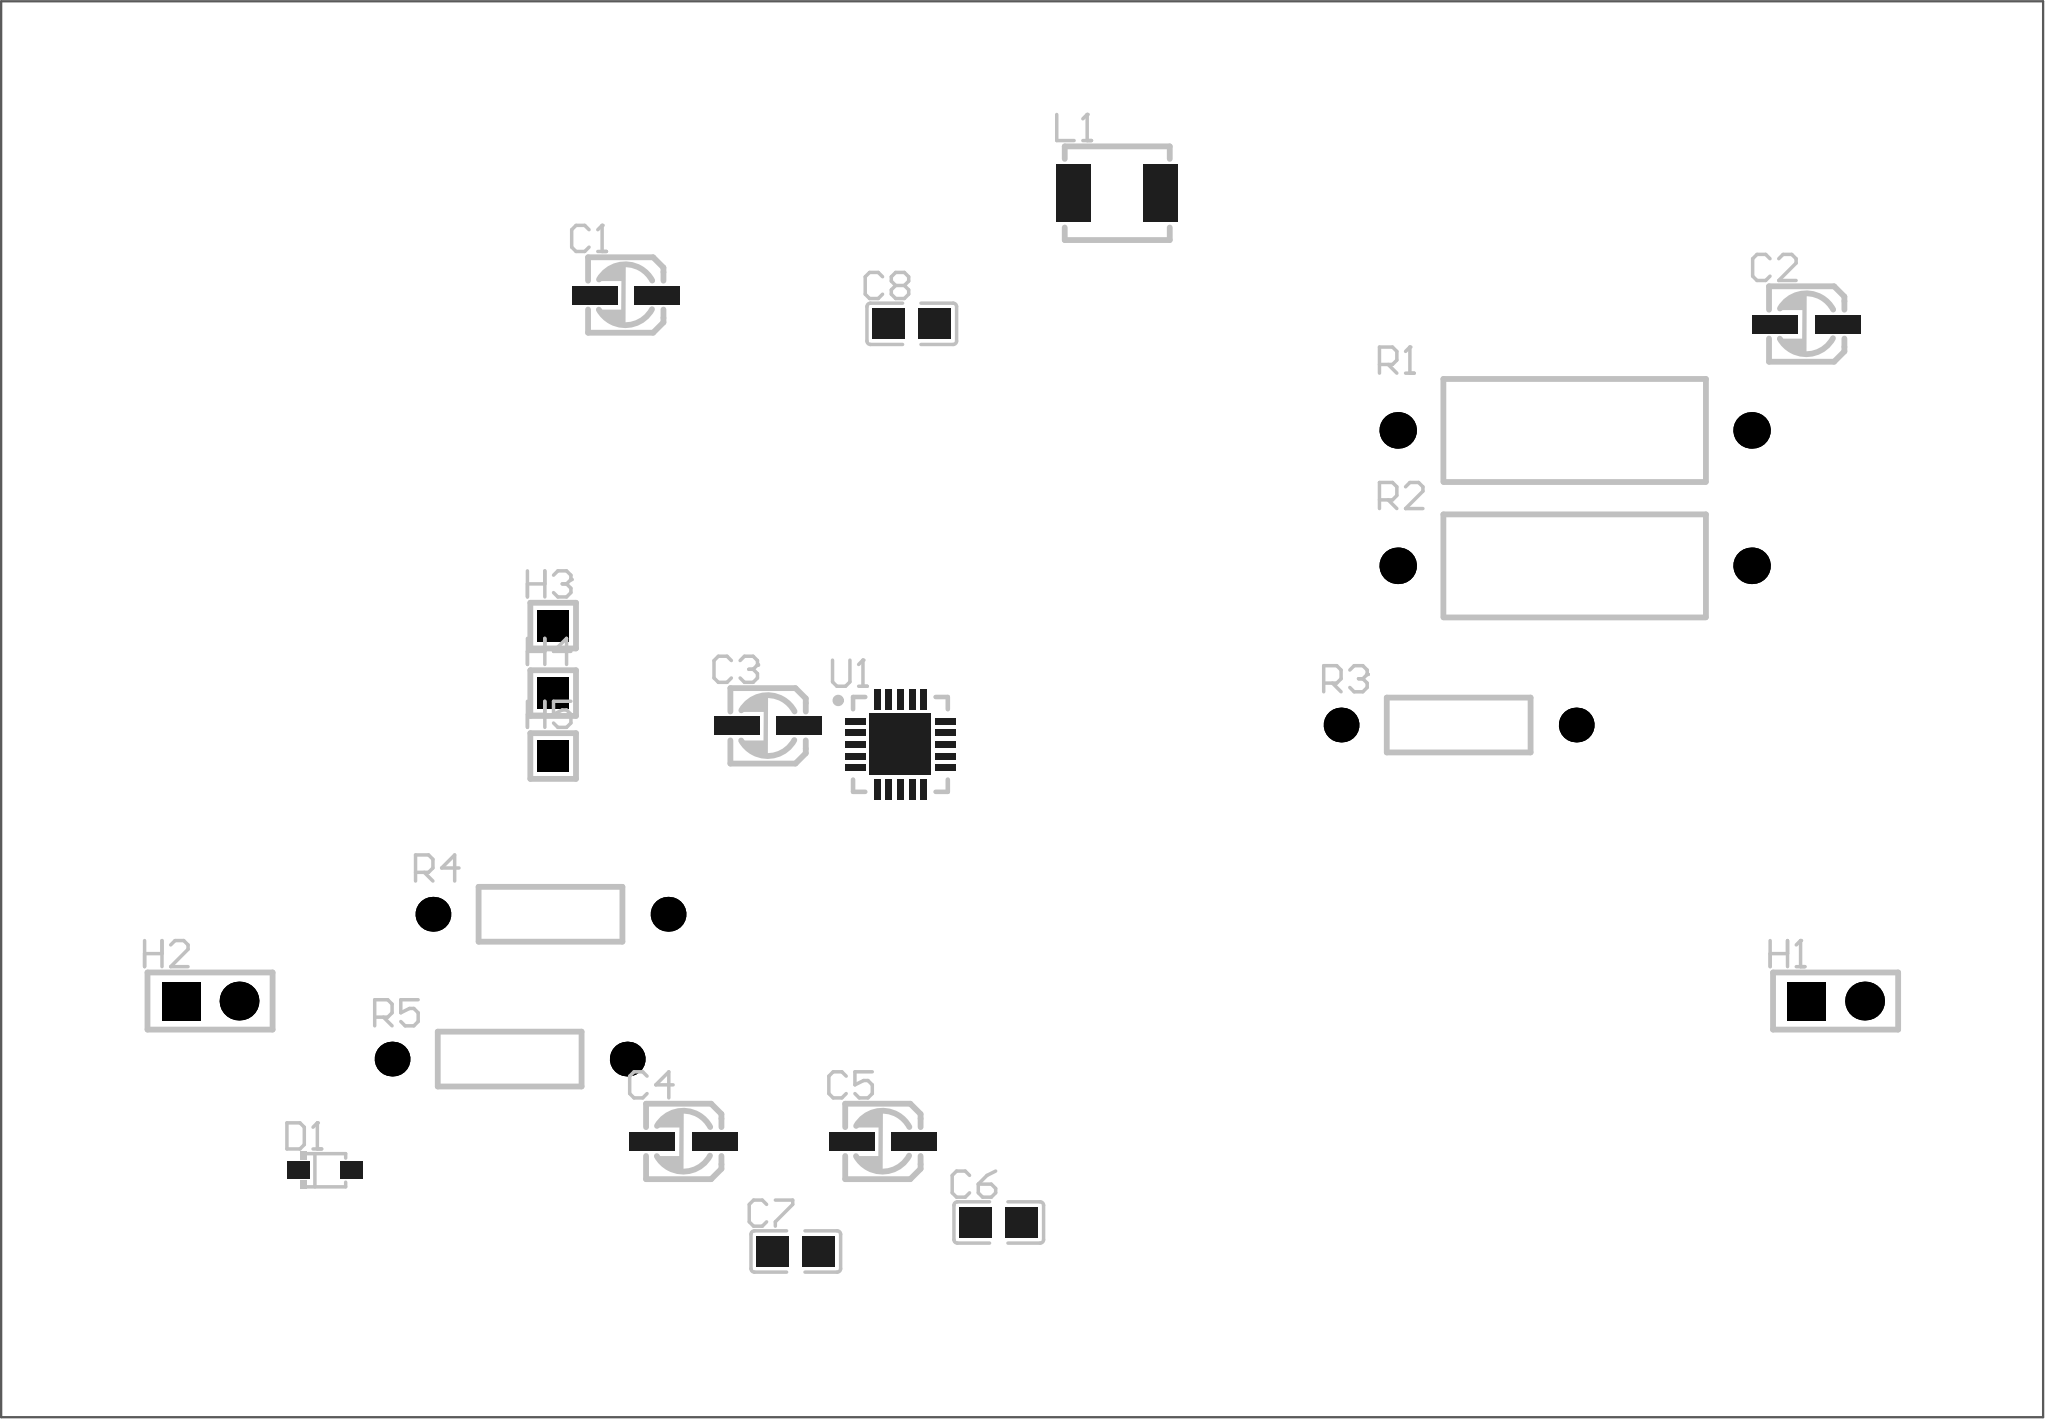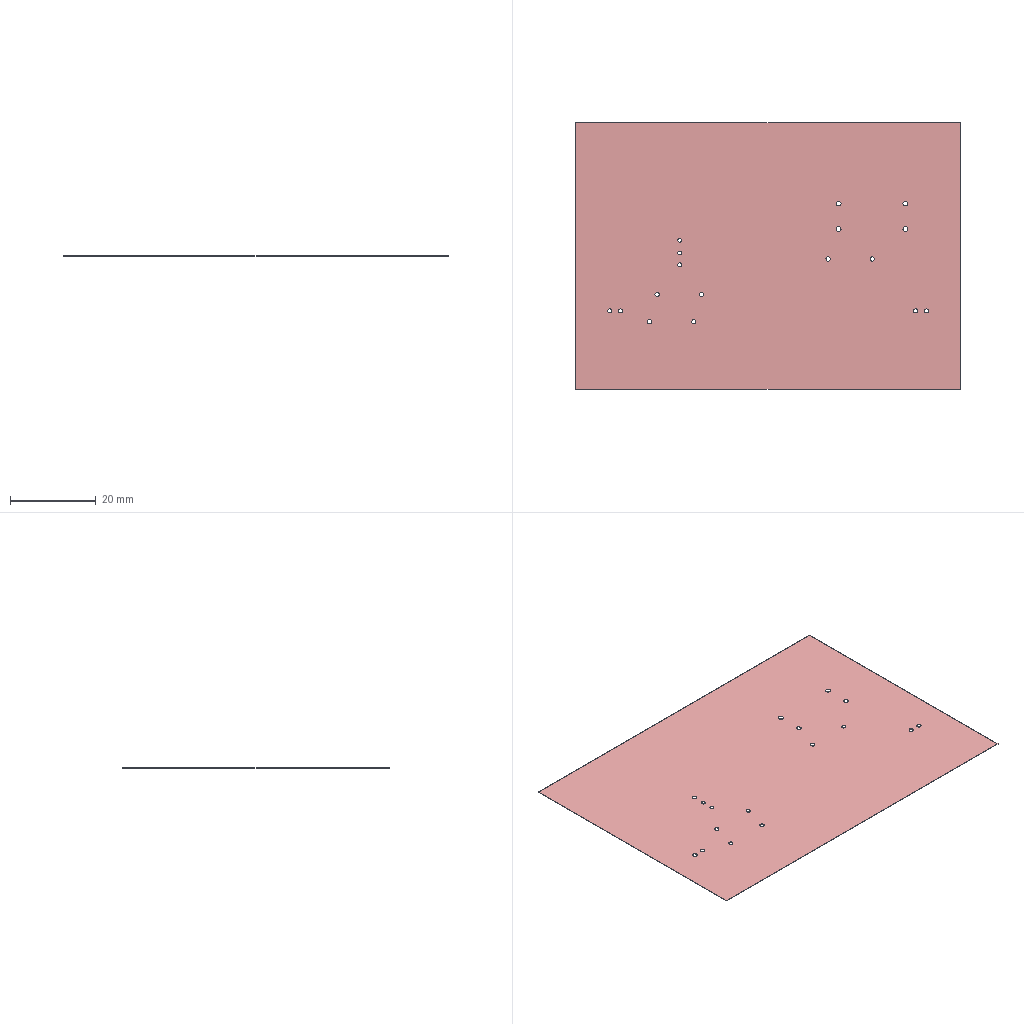Circuit board layout | Altium Designer | box 89.4 x 62 x 0.1 mm
Layer stack:
# Altium Designer layer stack of  (unit mm; dielectric type: 0 none, 1 core, 2 prepreg, 3 surface material)
index,name,kind,layer,copper_thickness_mm,dielectric_type,dielectric_thickness_mm,dielectric_material,dielectric_constant
0,Top Paste Mask Layer,other,,,,,,
1,Top Silkscreen Layer,other,,,,,,
2,Top Solder Mask Layer,dielectric,,,3,0.01,,3.3
3,Top Layer,copper,Top Layer,0.035,,,,
4,Bottom Layer,copper,Bottom Layer,0.035,,,,
5,Bottom Solder Mask Layer,dielectric,,,3,0.01,,3.3
6,Bottom Silkscreen Layer,other,,,,,,
7,Bottom Paste Mask Layer,other,,,,,,
# drill layer pairs: low layer,high layer
drill_pair,Top Layer,Bottom Layer
Part placement:
Designator,Comment,Layer,Footprint,Center-X(mm),Center-Y(mm),Rotation
C1,0.1uF,TopLayer,C_Ele_SMD_3x5.4mm,97.209,118.96,0
C2,100nF/250V,TopLayer,C_Ele_SMD_3x5.4mm,148.938,117.69,0
C3,0.1u,TopLayer,C_Ele_SMD_3x5.4mm,103.443,100.103,0
C4,10nF,TopLayer,C_Ele_SMD_3x5.4mm,99.749,81.914,0
C5,10nF,TopLayer,C_Ele_SMD_3x5.4mm,108.473,81.914,0
C6,100nF,TopLayer,C0805,113.548,78.374,0
C7,100nF,TopLayer,C0805,104.658,77.104,0
C8,10u,TopLayer,C0805,109.738,117.704,0
D1,BAT165E6327,TopLayer,SOD-323_L1.8-W1.3-LS2.5-RD,84.04,80.658,0
H1,,TopLayer,HDR-TH_2P-P2.54-V-F,150.203,88.064,0
H2,,TopLayer,HDR-TH_2P-P2.54-V-F,79,88.064,0
H3,,TopLayer,HDR-TH_1P-V-M_XKB_X4611WV-01I-C28D40,94.029,104.496,0
H4,,TopLayer,HDR-TH_1P-V-M_XKB_X4611WV-01I-C28D40,94.029,101.542,0
H5,,TopLayer,HDR-TH_1P-V-M_XKB_X4611WV-01I-C28D40,94.029,98.788,0
L1,4.7uH,TopLayer,IND-SMD_L4.6-W4.1-A,118.737,123.42,0
R1,1.72M,TopLayer,Res_1W,138.773,113.04,0
R2,15k,TopLayer,Res_1W,138.773,107.113,0
R3,18k,TopLayer,Res_1/4W,133.693,100.145,0
R4,1k,TopLayer,Res_1/4W,93.913,91.862,0
R5,1k,TopLayer,Res_1/4W,92.124,85.525,0
U1,DRV2700,TopLayer,TI-RGP20-2700X2700TP_V,109.24,99.296,0
Pad and via stacks:
# Altium Designer via and pad stacks of  (unit mm). Each distinct definition once, with the count of objects using it.
# via: kind,start_layer,end_layer,hole_mm,diameter_mm,mode(0 simple;1 top-mid-bottom;2 full stack),diameter_per_layer,count,example_net
# pad: kind,layer,hole_mm,hole_type(0 round;1 square;2 slot),plating,top_size,top_shape(1 round;2 rect;3 octagon;9 rounded rect),mid_size,bottom_size,mode,footprint,size_per_layer,count,example
pad,Top Layer,0,0,plated,1.999x0.8001,2,1.999x0.8001,1.999x0.8001,0,C_Ele_SMD_3x5.4mm,,10,C1.1
pad,Top Layer,0,0,plated,1.41x1.35,2,1.41x1.35,1.41x1.35,0,C0805,,6,C6.2
pad,Top Layer,0,0,plated,1x0.75,2,1x0.75,1x0.75,0,SOD-323_L1.8-W1.3-LS2.5-RD,,2,D1.2
pad,Top Layer,0,0,plated,2.5x1.5,2,2.5x1.5,2.5x1.5,0,IND-SMD_L4.6-W4.1-A,,2,L1.1
pad,Top Layer,0,0,plated,2.705x2.705,2,2.705x2.705,2.705x2.705,0,TI-RGP20-2700X2700TP_V,,1,U1.21
pad,Top Layer,0,0,plated,0.2921x0.8763,2,0.2921x0.8763,0.2921x0.8763,0,TI-RGP20-2700X2700TP_V,,20,U1.20
pad,Multi-Layer,1,0,plated,1.7x1.7,2,1.7x1.7,1.7x1.7,0,HDR-TH_2P-P2.54-V-F,,2,H1.1
pad,Multi-Layer,1,0,plated,1.7x1.7,1,1.7x1.7,1.7x1.7,0,HDR-TH_2P-P2.54-V-F,,2,H1.2
pad,Multi-Layer,0.9,0,plated,1.4x1.4,2,1.4x1.4,1.4x1.4,0,HDR-TH_1P-V-M_XKB_X4611WV-01I-C28D40,,3,H3.1
pad,Multi-Layer,1.1,0,plated,1.6x1.6,1,1.6x1.6,1.6x1.6,0,Res_1W,,4,R1.1
pad,Multi-Layer,1,0,plated,1.524x1.524,1,1.524x1.524,1.524x1.524,0,Res_1/4W,,6,R3.1
via,Top Layer,Bottom Layer,0.2997,0.5004,0,,9,GND
Design rules, without the lines most boards share:
# Altium Designer design rules of  (exported by Altium Designer, unit mm)
# columns: name | kind | enabled | priority | scope1 | scope2 | descriptor | typed fields (field=value)
Plane_innerPlane | 0 | disabled | 1 | All | All | Clearance Constraint (Gap=6mil) (Disabled)(All),(All) | gap=0.1524
Plane_innerPlane_1 | 63 | disabled | 1 | All | All | Board Clearance Constraint (Gap=0mil) (Disabled)(All) |
Copper_copperRegion | 0 | disabled | 2 | All | All | Clearance Constraint (Gap=6mil) (Disabled)(All),(All) | gap=0.1524
Copper_copperRegion_1 | 63 | disabled | 2 | All | All | Board Clearance Constraint (Gap=0mil) (Disabled)(All) |
copperThickness1oz | 0 | enabled | 3 | All | All | Clearance Constraint (Gap=6mil) (All),(All) | gap=0.1524
copperThickness1oz_1 | 63 | enabled | 3 | All | All | Board Clearance Constraint (Gap=0mil) (All) |
otherClearance | 52 | enabled | 1 | All | All | Hole To Hole Clearance (Gap=11.8mil) (All),(All) | gap=0.2997
copperThickness1oz_2 | 2 | enabled | 1 | All | All | Width Constraint (Min=5mil) (Max=100mil) (Preferred=10mil) (All) |
differentialPair | 51 | enabled | 1 | All | All | Differential Pairs Uncoupled Length using the Gap Constraints (Min=5mil) (Max=6mil) (Prefered=6mil)  and Width Constraints (Min=5mil) (Max=100mil) (Prefered=100mil) (All) |
viaSize | 11 | enabled | 1 | All | All | Routing Via (MinHoleWidth=19.7mil) (MaxHoleWidth=393.7mil) (PreferredHoleWidth=24mil) (MinWidth=11.8mil) (MaxWidth=248mil) (PreferedWidth=12mil) (All) | via_min_hole=0.5004 via_max_hole=10 via_preferred_diameter=0.3048 via_preferred_hole=0.6096